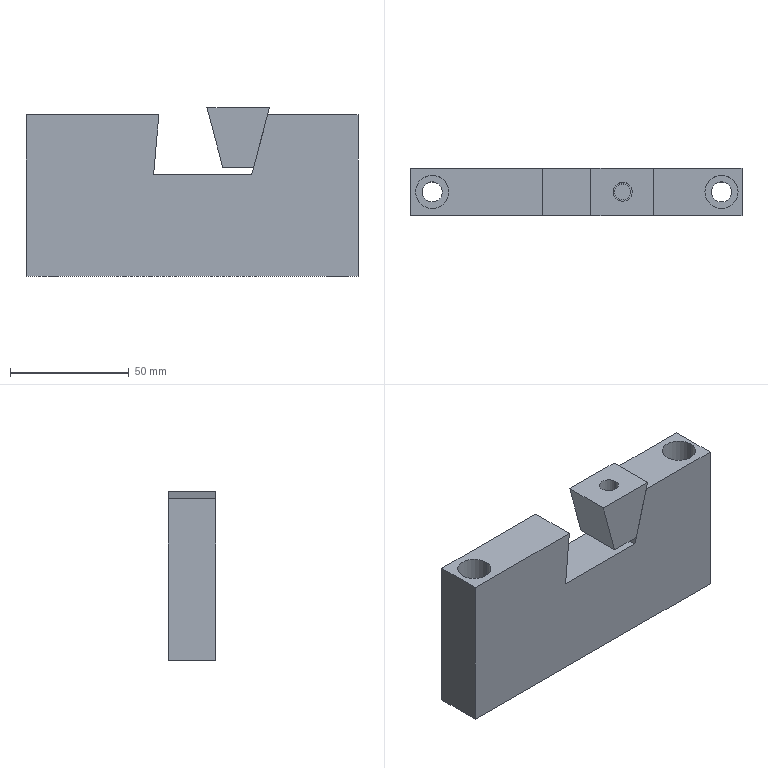Part | Mastercam | 2 solids | 31 faces | box 140 x 20 x 71 mm | volume 164195 mm3 | plane 19 | cylinder 12 | commonest cylinder face diameters 8.5 x4 14 x4 6.8 x2 8 x2
STEP:
#1=CARTESIAN_POINT('',(0.,0.,0.));
#2=DIRECTION('',(0.,0.,1.));
#3=DIRECTION('',(1.,0.,0.));
#4=AXIS2_PLACEMENT_3D('',#1,#2,#3);
#5=CARTESIAN_POINT('',(26.175,18.5,-9.5));
#6=VERTEX_POINT('',#5);
#7=CARTESIAN_POINT('',(18.175,18.5,-9.5));
#8=VERTEX_POINT('',#7);
#9=CARTESIAN_POINT('',(22.175,18.5,-9.5));
#10=DIRECTION('',(0.,0.,-1.));
#11=DIRECTION('',(-1.,0.,0.));
#12=AXIS2_PLACEMENT_3D('',#9,#10,#11);
#13=CIRCLE('',#12,4.);
#14=EDGE_CURVE('',#6,#8,#13,.T.);
#15=ORIENTED_EDGE('',*,*,#14,.F.);
#16=CARTESIAN_POINT('',(22.175,18.5,-9.5));
#17=DIRECTION('',(0.,0.,-1.));
#18=DIRECTION('',(-1.,0.,0.));
#19=AXIS2_PLACEMENT_3D('',#16,#17,#18);
#20=CIRCLE('',#19,4.);
#21=EDGE_CURVE('',#8,#6,#20,.T.);
#22=ORIENTED_EDGE('',*,*,#21,.F.);
#23=EDGE_LOOP('',(#15,#22));
#24=FACE_BOUND('',#23,.T.);
#25=CARTESIAN_POINT('',(15.485,28.5,-9.5));
#26=VERTEX_POINT('',#25);
#27=CARTESIAN_POINT('',(28.476,28.5,-9.5));
#28=VERTEX_POINT('',#27);
#29=CARTESIAN_POINT('',(16.735,28.5,-9.5));
#30=DIRECTION('',(1.,0.,0.));
#31=VECTOR('',#30,1.);
#32=LINE('',#29,#31);
#33=EDGE_CURVE('',#26,#28,#32,.T.);
#34=ORIENTED_EDGE('',*,*,#33,.T.);
#35=CARTESIAN_POINT('',(28.476,8.5,-9.5));
#36=VERTEX_POINT('',#35);
#37=CARTESIAN_POINT('',(28.476,28.5,-9.5));
#38=DIRECTION('',(0.,-1.,0.));
#39=VECTOR('',#38,1.);
#40=LINE('',#37,#39);
#41=EDGE_CURVE('',#28,#36,#40,.T.);
#42=ORIENTED_EDGE('',*,*,#41,.T.);
#43=CARTESIAN_POINT('',(15.485,8.5,-9.5));
#44=VERTEX_POINT('',#43);
#45=CARTESIAN_POINT('',(16.735,8.5,-9.5));
#46=DIRECTION('',(1.,0.,0.));
#47=VECTOR('',#46,1.);
#48=LINE('',#45,#47);
#49=EDGE_CURVE('',#44,#36,#48,.T.);
#50=ORIENTED_EDGE('',*,*,#49,.F.);
#51=CARTESIAN_POINT('',(15.485,28.5,-9.5));
#52=DIRECTION('',(0.,-1.,0.));
#53=VECTOR('',#52,1.);
#54=LINE('',#51,#53);
#55=EDGE_CURVE('',#26,#44,#54,.T.);
#56=ORIENTED_EDGE('',*,*,#55,.F.);
#57=EDGE_LOOP('',(#34,#42,#50,#56));
#58=FACE_OUTER_BOUND('',#57,.T.);
#59=CARTESIAN_POINT('',(16.735,28.5,-9.5));
#60=DIRECTION('',(0.,0.,-1.));
#61=DIRECTION('',(-1.,0.,0.));
#62=AXIS2_PLACEMENT_3D('',#59,#60,#61);
#63=PLANE('',#62);
#64=ADVANCED_FACE('',(#24,#58),#63,.T.);
#65=CARTESIAN_POINT('',(8.786,28.5,15.5));
#66=VERTEX_POINT('',#65);
#67=CARTESIAN_POINT('',(35.175,28.5,15.5));
#68=VERTEX_POINT('',#67);
#69=CARTESIAN_POINT('',(12.68,28.5,15.5));
#70=DIRECTION('',(1.,0.,0.));
#71=VECTOR('',#70,1.);
#72=LINE('',#69,#71);
#73=EDGE_CURVE('',#66,#68,#72,.T.);
#74=ORIENTED_EDGE('',*,*,#73,.T.);
#75=CARTESIAN_POINT('',(28.432,28.5,-9.665));
#76=DIRECTION('',(-0.2588,0.,-0.9659));
#77=VECTOR('',#76,1.);
#78=LINE('',#75,#77);
#79=EDGE_CURVE('',#68,#28,#78,.T.);
#80=ORIENTED_EDGE('',*,*,#79,.T.);
#81=ORIENTED_EDGE('',*,*,#33,.F.);
#82=CARTESIAN_POINT('',(17.578,28.5,-17.312));
#83=DIRECTION('',(-0.2588,0.,0.9659));
#84=VECTOR('',#83,1.);
#85=LINE('',#82,#84);
#86=EDGE_CURVE('',#26,#66,#85,.T.);
#87=ORIENTED_EDGE('',*,*,#86,.T.);
#88=EDGE_LOOP('',(#74,#80,#81,#87));
#89=FACE_OUTER_BOUND('',#88,.T.);
#90=CARTESIAN_POINT('',(-1.,28.5,-4.5));
#91=DIRECTION('',(0.,1.,0.));
#92=DIRECTION('',(0.,0.,1.));
#93=AXIS2_PLACEMENT_3D('',#90,#91,#92);
#94=PLANE('',#93);
#95=ADVANCED_FACE('',(#89),#94,.T.);
#96=CARTESIAN_POINT('',(35.175,8.5,15.5));
#97=VERTEX_POINT('',#96);
#98=CARTESIAN_POINT('',(26.405,8.5,-17.232));
#99=DIRECTION('',(0.2588,0.,0.9659));
#100=VECTOR('',#99,1.);
#101=LINE('',#98,#100);
#102=EDGE_CURVE('',#36,#97,#101,.T.);
#103=ORIENTED_EDGE('',*,*,#102,.T.);
#104=CARTESIAN_POINT('',(8.786,8.5,15.5));
#105=VERTEX_POINT('',#104);
#106=CARTESIAN_POINT('',(12.68,8.5,15.5));
#107=DIRECTION('',(1.,0.,0.));
#108=VECTOR('',#107,1.);
#109=LINE('',#106,#108);
#110=EDGE_CURVE('',#105,#97,#109,.T.);
#111=ORIENTED_EDGE('',*,*,#110,.F.);
#112=CARTESIAN_POINT('',(17.578,8.5,-17.312));
#113=DIRECTION('',(-0.2588,0.,0.9659));
#114=VECTOR('',#113,1.);
#115=LINE('',#112,#114);
#116=EDGE_CURVE('',#44,#105,#115,.T.);
#117=ORIENTED_EDGE('',*,*,#116,.F.);
#118=ORIENTED_EDGE('',*,*,#49,.T.);
#119=EDGE_LOOP('',(#103,#111,#117,#118));
#120=FACE_OUTER_BOUND('',#119,.T.);
#121=CARTESIAN_POINT('',(-1.,8.5,-4.5));
#122=DIRECTION('',(0.,1.,0.));
#123=DIRECTION('',(0.,0.,1.));
#124=AXIS2_PLACEMENT_3D('',#121,#122,#123);
#125=PLANE('',#124);
#126=ADVANCED_FACE('',(#120),#125,.F.);
#127=CARTESIAN_POINT('',(26.175,18.5,15.5));
#128=VERTEX_POINT('',#127);
#129=CARTESIAN_POINT('',(18.175,18.5,15.5));
#130=VERTEX_POINT('',#129);
#131=CARTESIAN_POINT('',(22.175,18.5,15.5));
#132=DIRECTION('',(0.,0.,1.));
#133=DIRECTION('',(-1.,0.,0.));
#134=AXIS2_PLACEMENT_3D('',#131,#132,#133);
#135=CIRCLE('',#134,4.);
#136=EDGE_CURVE('',#128,#130,#135,.T.);
#137=ORIENTED_EDGE('',*,*,#136,.F.);
#138=CARTESIAN_POINT('',(22.175,18.5,15.5));
#139=DIRECTION('',(0.,0.,1.));
#140=DIRECTION('',(-1.,0.,0.));
#141=AXIS2_PLACEMENT_3D('',#138,#139,#140);
#142=CIRCLE('',#141,4.);
#143=EDGE_CURVE('',#130,#128,#142,.T.);
#144=ORIENTED_EDGE('',*,*,#143,.F.);
#145=EDGE_LOOP('',(#137,#144));
#146=FACE_BOUND('',#145,.T.);
#147=ORIENTED_EDGE('',*,*,#110,.T.);
#148=CARTESIAN_POINT('',(35.175,28.5,15.5));
#149=DIRECTION('',(0.,-1.,0.));
#150=VECTOR('',#149,1.);
#151=LINE('',#148,#150);
#152=EDGE_CURVE('',#68,#97,#151,.T.);
#153=ORIENTED_EDGE('',*,*,#152,.F.);
#154=ORIENTED_EDGE('',*,*,#73,.F.);
#155=CARTESIAN_POINT('',(8.786,28.5,15.5));
#156=DIRECTION('',(0.,-1.,0.));
#157=VECTOR('',#156,1.);
#158=LINE('',#155,#157);
#159=EDGE_CURVE('',#66,#105,#158,.T.);
#160=ORIENTED_EDGE('',*,*,#159,.T.);
#161=EDGE_LOOP('',(#147,#153,#154,#160));
#162=FACE_OUTER_BOUND('',#161,.T.);
#163=CARTESIAN_POINT('',(12.68,28.5,15.5));
#164=DIRECTION('',(0.,0.,-1.));
#165=DIRECTION('',(-1.,0.,0.));
#166=AXIS2_PLACEMENT_3D('',#163,#164,#165);
#167=PLANE('',#166);
#168=ADVANCED_FACE('',(#146,#162),#167,.F.);
#169=ORIENTED_EDGE('',*,*,#116,.T.);
#170=ORIENTED_EDGE('',*,*,#159,.F.);
#171=ORIENTED_EDGE('',*,*,#86,.F.);
#172=ORIENTED_EDGE('',*,*,#55,.T.);
#173=EDGE_LOOP('',(#169,#170,#171,#172));
#174=FACE_OUTER_BOUND('',#173,.T.);
#175=CARTESIAN_POINT('',(17.578,28.5,-17.312));
#176=DIRECTION('',(0.9659,0.,0.2588));
#177=DIRECTION('',(0.2588,0.,-0.9659));
#178=AXIS2_PLACEMENT_3D('',#175,#176,#177);
#179=PLANE('',#178);
#180=ADVANCED_FACE('',(#174),#179,.F.);
#181=CARTESIAN_POINT('',(18.175,18.5,-9.5));
#182=DIRECTION('',(0.,0.,1.));
#183=VECTOR('',#182,1.);
#184=LINE('',#181,#183);
#185=EDGE_CURVE('',#8,#130,#184,.T.);
#186=ORIENTED_EDGE('',*,*,#185,.T.);
#187=ORIENTED_EDGE('',*,*,#143,.T.);
#188=CARTESIAN_POINT('',(26.175,18.5,-9.5));
#189=DIRECTION('',(0.,0.,1.));
#190=VECTOR('',#189,1.);
#191=LINE('',#188,#190);
#192=EDGE_CURVE('',#6,#128,#191,.T.);
#193=ORIENTED_EDGE('',*,*,#192,.F.);
#194=ORIENTED_EDGE('',*,*,#14,.T.);
#195=EDGE_LOOP('',(#186,#187,#193,#194));
#196=FACE_OUTER_BOUND('',#195,.T.);
#197=CARTESIAN_POINT('',(22.175,18.5,-17.51));
#198=DIRECTION('',(0.,0.,1.));
#199=DIRECTION('',(0.,1.,0.));
#200=AXIS2_PLACEMENT_3D('',#197,#198,#199);
#201=CYLINDRICAL_SURFACE('',#200,4.);
#202=ADVANCED_FACE('',(#196),#201,.F.);
#203=ORIENTED_EDGE('',*,*,#152,.T.);
#204=ORIENTED_EDGE('',*,*,#102,.F.);
#205=ORIENTED_EDGE('',*,*,#41,.F.);
#206=ORIENTED_EDGE('',*,*,#79,.F.);
#207=EDGE_LOOP('',(#203,#204,#205,#206));
#208=FACE_OUTER_BOUND('',#207,.T.);
#209=CARTESIAN_POINT('',(26.405,31.5,-17.232));
#210=DIRECTION('',(0.9659,0.,-0.2588));
#211=DIRECTION('',(-0.2588,0.,-0.9659));
#212=AXIS2_PLACEMENT_3D('',#209,#210,#211);
#213=PLANE('',#212);
#214=ADVANCED_FACE('',(#208),#213,.T.);
#215=ORIENTED_EDGE('',*,*,#185,.F.);
#216=ORIENTED_EDGE('',*,*,#21,.T.);
#217=ORIENTED_EDGE('',*,*,#192,.T.);
#218=ORIENTED_EDGE('',*,*,#136,.T.);
#219=EDGE_LOOP('',(#215,#216,#217,#218));
#220=FACE_OUTER_BOUND('',#219,.T.);
#221=CARTESIAN_POINT('',(22.175,18.5,-17.51));
#222=DIRECTION('',(0.,0.,1.));
#223=DIRECTION('',(0.,-1.,0.));
#224=AXIS2_PLACEMENT_3D('',#221,#222,#223);
#225=CYLINDRICAL_SURFACE('',#224,4.);
#226=ADVANCED_FACE('',(#220),#225,.F.);
#227=CLOSED_SHELL('',(#64,#95,#126,#168,#180,#202,#214,#226));
#228=MANIFOLD_SOLID_BREP('',#227);
#229=CARTESIAN_POINT('',(18.775,18.5,-12.5));
#230=VERTEX_POINT('',#229);
#231=CARTESIAN_POINT('',(25.575,18.5,-12.5));
#232=VERTEX_POINT('',#231);
#233=CARTESIAN_POINT('',(22.175,18.5,-12.5));
#234=DIRECTION('',(0.,0.,-1.));
#235=DIRECTION('',(-1.,0.,0.));
#236=AXIS2_PLACEMENT_3D('',#233,#234,#235);
#237=CIRCLE('',#236,3.4);
#238=EDGE_CURVE('',#230,#232,#237,.T.);
#239=ORIENTED_EDGE('',*,*,#238,.T.);
#240=CARTESIAN_POINT('',(22.175,18.5,-12.5));
#241=DIRECTION('',(0.,0.,-1.));
#242=DIRECTION('',(-1.,0.,0.));
#243=AXIS2_PLACEMENT_3D('',#240,#241,#242);
#244=CIRCLE('',#243,3.4);
#245=EDGE_CURVE('',#232,#230,#244,.T.);
#246=ORIENTED_EDGE('',*,*,#245,.T.);
#247=EDGE_LOOP('',(#239,#246));
#248=FACE_BOUND('',#247,.T.);
#249=CARTESIAN_POINT('',(27.673,28.5,-12.5));
#250=VERTEX_POINT('',#249);
#251=CARTESIAN_POINT('',(27.673,8.5,-12.5));
#252=VERTEX_POINT('',#251);
#253=CARTESIAN_POINT('',(27.673,58.5,-12.5));
#254=DIRECTION('',(0.,-1.,0.));
#255=VECTOR('',#254,1.);
#256=LINE('',#253,#255);
#257=EDGE_CURVE('',#250,#252,#256,.T.);
#258=ORIENTED_EDGE('',*,*,#257,.F.);
#259=CARTESIAN_POINT('',(-13.683,28.5,-12.5));
#260=VERTEX_POINT('',#259);
#261=CARTESIAN_POINT('',(-20.5,28.5,-12.5));
#262=DIRECTION('',(1.,0.,0.));
#263=VECTOR('',#262,1.);
#264=LINE('',#261,#263);
#265=EDGE_CURVE('',#260,#250,#264,.T.);
#266=ORIENTED_EDGE('',*,*,#265,.F.);
#267=CARTESIAN_POINT('',(-13.683,8.5,-12.5));
#268=VERTEX_POINT('',#267);
#269=CARTESIAN_POINT('',(-13.683,33.5,-12.5));
#270=DIRECTION('',(0.,-1.,0.));
#271=VECTOR('',#270,1.);
#272=LINE('',#269,#271);
#273=EDGE_CURVE('',#260,#268,#272,.T.);
#274=ORIENTED_EDGE('',*,*,#273,.T.);
#275=CARTESIAN_POINT('',(-20.5,8.5,-12.5));
#276=DIRECTION('',(1.,0.,0.));
#277=VECTOR('',#276,1.);
#278=LINE('',#275,#277);
#279=EDGE_CURVE('',#268,#252,#278,.T.);
#280=ORIENTED_EDGE('',*,*,#279,.T.);
#281=EDGE_LOOP('',(#258,#266,#274,#280));
#282=FACE_OUTER_BOUND('',#281,.T.);
#283=CARTESIAN_POINT('',(-20.5,58.5,-12.5));
#284=DIRECTION('',(0.,0.,-1.));
#285=DIRECTION('',(-1.,0.,0.));
#286=AXIS2_PLACEMENT_3D('',#283,#284,#285);
#287=PLANE('',#286);
#288=ADVANCED_FACE('',(#248,#282),#287,.F.);
#289=CARTESIAN_POINT('',(-62.4,18.5,-55.5));
#290=VERTEX_POINT('',#289);
#291=CARTESIAN_POINT('',(-62.4,18.5,-10.5));
#292=VERTEX_POINT('',#291);
#293=CARTESIAN_POINT('',(-62.4,18.5,-55.5));
#294=DIRECTION('',(0.,0.,1.));
#295=VECTOR('',#294,1.);
#296=LINE('',#293,#295);
#297=EDGE_CURVE('',#290,#292,#296,.T.);
#298=ORIENTED_EDGE('',*,*,#297,.T.);
#299=CARTESIAN_POINT('',(-53.9,18.5,-10.5));
#300=VERTEX_POINT('',#299);
#301=CARTESIAN_POINT('',(-58.15,18.5,-10.5));
#302=DIRECTION('',(0.,0.,-1.));
#303=DIRECTION('',(1.,0.,0.));
#304=AXIS2_PLACEMENT_3D('',#301,#302,#303);
#305=CIRCLE('',#304,4.25);
#306=EDGE_CURVE('',#300,#292,#305,.T.);
#307=ORIENTED_EDGE('',*,*,#306,.F.);
#308=CARTESIAN_POINT('',(-53.9,18.5,-55.5));
#309=VERTEX_POINT('',#308);
#310=CARTESIAN_POINT('',(-53.9,18.5,-55.5));
#311=DIRECTION('',(0.,0.,1.));
#312=VECTOR('',#311,1.);
#313=LINE('',#310,#312);
#314=EDGE_CURVE('',#309,#300,#313,.T.);
#315=ORIENTED_EDGE('',*,*,#314,.F.);
#316=CARTESIAN_POINT('',(-58.15,18.5,-55.5));
#317=DIRECTION('',(0.,0.,1.));
#318=DIRECTION('',(1.,0.,0.));
#319=AXIS2_PLACEMENT_3D('',#316,#317,#318);
#320=CIRCLE('',#319,4.25);
#321=EDGE_CURVE('',#290,#309,#320,.T.);
#322=ORIENTED_EDGE('',*,*,#321,.F.);
#323=EDGE_LOOP('',(#298,#307,#315,#322));
#324=FACE_OUTER_BOUND('',#323,.T.);
#325=CARTESIAN_POINT('',(-58.15,18.5,-55.51));
#326=DIRECTION('',(0.,0.,1.));
#327=DIRECTION('',(0.,1.,0.));
#328=AXIS2_PLACEMENT_3D('',#325,#326,#327);
#329=CYLINDRICAL_SURFACE('',#328,4.25);
#330=ADVANCED_FACE('',(#324),#329,.F.);
#331=CARTESIAN_POINT('',(59.6,18.5,-55.5));
#332=VERTEX_POINT('',#331);
#333=CARTESIAN_POINT('',(59.6,18.5,-10.5));
#334=VERTEX_POINT('',#333);
#335=CARTESIAN_POINT('',(59.6,18.5,-55.5));
#336=DIRECTION('',(0.,0.,1.));
#337=VECTOR('',#336,1.);
#338=LINE('',#335,#337);
#339=EDGE_CURVE('',#332,#334,#338,.T.);
#340=ORIENTED_EDGE('',*,*,#339,.T.);
#341=CARTESIAN_POINT('',(68.1,18.5,-10.5));
#342=VERTEX_POINT('',#341);
#343=CARTESIAN_POINT('',(63.85,18.5,-10.5));
#344=DIRECTION('',(0.,0.,-1.));
#345=DIRECTION('',(1.,0.,0.));
#346=AXIS2_PLACEMENT_3D('',#343,#344,#345);
#347=CIRCLE('',#346,4.25);
#348=EDGE_CURVE('',#342,#334,#347,.T.);
#349=ORIENTED_EDGE('',*,*,#348,.F.);
#350=CARTESIAN_POINT('',(68.1,18.5,-55.5));
#351=VERTEX_POINT('',#350);
#352=CARTESIAN_POINT('',(68.1,18.5,-55.5));
#353=DIRECTION('',(0.,0.,1.));
#354=VECTOR('',#353,1.);
#355=LINE('',#352,#354);
#356=EDGE_CURVE('',#351,#342,#355,.T.);
#357=ORIENTED_EDGE('',*,*,#356,.F.);
#358=CARTESIAN_POINT('',(63.85,18.5,-55.5));
#359=DIRECTION('',(0.,0.,1.));
#360=DIRECTION('',(1.,0.,0.));
#361=AXIS2_PLACEMENT_3D('',#358,#359,#360);
#362=CIRCLE('',#361,4.25);
#363=EDGE_CURVE('',#332,#351,#362,.T.);
#364=ORIENTED_EDGE('',*,*,#363,.F.);
#365=EDGE_LOOP('',(#340,#349,#357,#364));
#366=FACE_OUTER_BOUND('',#365,.T.);
#367=CARTESIAN_POINT('',(63.85,18.5,-55.51));
#368=DIRECTION('',(0.,0.,1.));
#369=DIRECTION('',(0.,1.,0.));
#370=AXIS2_PLACEMENT_3D('',#367,#368,#369);
#371=CYLINDRICAL_SURFACE('',#370,4.25);
#372=ADVANCED_FACE('',(#366),#371,.F.);
#373=CARTESIAN_POINT('',(-67.5,8.5,12.5));
#374=VERTEX_POINT('',#373);
#375=CARTESIAN_POINT('',(-67.5,8.5,-55.5));
#376=VERTEX_POINT('',#375);
#377=CARTESIAN_POINT('',(-67.5,8.5,12.5));
#378=DIRECTION('',(0.,0.,-1.));
#379=VECTOR('',#378,1.);
#380=LINE('',#377,#379);
#381=EDGE_CURVE('',#374,#376,#380,.T.);
#382=ORIENTED_EDGE('',*,*,#381,.F.);
#383=CARTESIAN_POINT('',(-67.5,28.5,12.5));
#384=VERTEX_POINT('',#383);
#385=CARTESIAN_POINT('',(-67.5,58.5,12.5));
#386=DIRECTION('',(0.,-1.,0.));
#387=VECTOR('',#386,1.);
#388=LINE('',#385,#387);
#389=EDGE_CURVE('',#384,#374,#388,.T.);
#390=ORIENTED_EDGE('',*,*,#389,.F.);
#391=CARTESIAN_POINT('',(-67.5,28.5,-55.5));
#392=VERTEX_POINT('',#391);
#393=CARTESIAN_POINT('',(-67.5,28.5,12.5));
#394=DIRECTION('',(0.,0.,-1.));
#395=VECTOR('',#394,1.);
#396=LINE('',#393,#395);
#397=EDGE_CURVE('',#384,#392,#396,.T.);
#398=ORIENTED_EDGE('',*,*,#397,.T.);
#399=CARTESIAN_POINT('',(-67.5,58.5,-55.5));
#400=DIRECTION('',(0.,-1.,0.));
#401=VECTOR('',#400,1.);
#402=LINE('',#399,#401);
#403=EDGE_CURVE('',#392,#376,#402,.T.);
#404=ORIENTED_EDGE('',*,*,#403,.T.);
#405=EDGE_LOOP('',(#382,#390,#398,#404));
#406=FACE_OUTER_BOUND('',#405,.T.);
#407=CARTESIAN_POINT('',(-67.5,58.5,12.5));
#408=DIRECTION('',(-1.,0.,0.));
#409=DIRECTION('',(0.,0.,1.));
#410=AXIS2_PLACEMENT_3D('',#407,#408,#409);
#411=PLANE('',#410);
#412=ADVANCED_FACE('',(#406),#411,.T.);
#413=CARTESIAN_POINT('',(-58.15,18.5,-55.5));
#414=DIRECTION('',(0.,0.,1.));
#415=DIRECTION('',(1.,0.,0.));
#416=AXIS2_PLACEMENT_3D('',#413,#414,#415);
#417=CIRCLE('',#416,4.25);
#418=EDGE_CURVE('',#309,#290,#417,.T.);
#419=ORIENTED_EDGE('',*,*,#418,.T.);
#420=ORIENTED_EDGE('',*,*,#321,.T.);
#421=EDGE_LOOP('',(#419,#420));
#422=FACE_BOUND('',#421,.T.);
#423=CARTESIAN_POINT('',(63.85,18.5,-55.5));
#424=DIRECTION('',(0.,0.,1.));
#425=DIRECTION('',(1.,0.,0.));
#426=AXIS2_PLACEMENT_3D('',#423,#424,#425);
#427=CIRCLE('',#426,4.25);
#428=EDGE_CURVE('',#351,#332,#427,.T.);
#429=ORIENTED_EDGE('',*,*,#428,.T.);
#430=ORIENTED_EDGE('',*,*,#363,.T.);
#431=EDGE_LOOP('',(#429,#430));
#432=FACE_BOUND('',#431,.T.);
#433=CARTESIAN_POINT('',(72.5,8.5,-55.5));
#434=VERTEX_POINT('',#433);
#435=CARTESIAN_POINT('',(41.2,8.5,-55.5));
#436=DIRECTION('',(-1.,0.,0.));
#437=VECTOR('',#436,1.);
#438=LINE('',#435,#437);
#439=EDGE_CURVE('',#434,#376,#438,.T.);
#440=ORIENTED_EDGE('',*,*,#439,.T.);
#441=ORIENTED_EDGE('',*,*,#403,.F.);
#442=CARTESIAN_POINT('',(72.5,28.5,-55.5));
#443=VERTEX_POINT('',#442);
#444=CARTESIAN_POINT('',(41.2,28.5,-55.5));
#445=DIRECTION('',(-1.,0.,0.));
#446=VECTOR('',#445,1.);
#447=LINE('',#444,#446);
#448=EDGE_CURVE('',#443,#392,#447,.T.);
#449=ORIENTED_EDGE('',*,*,#448,.F.);
#450=CARTESIAN_POINT('',(72.5,58.5,-55.5));
#451=DIRECTION('',(0.,-1.,0.));
#452=VECTOR('',#451,1.);
#453=LINE('',#450,#452);
#454=EDGE_CURVE('',#443,#434,#453,.T.);
#455=ORIENTED_EDGE('',*,*,#454,.T.);
#456=EDGE_LOOP('',(#440,#441,#449,#455));
#457=FACE_OUTER_BOUND('',#456,.T.);
#458=CARTESIAN_POINT('',(41.2,58.5,-55.5));
#459=DIRECTION('',(0.,0.,1.));
#460=DIRECTION('',(1.,0.,0.));
#461=AXIS2_PLACEMENT_3D('',#458,#459,#460);
#462=PLANE('',#461);
#463=ADVANCED_FACE('',(#422,#432,#457),#462,.F.);
#464=CARTESIAN_POINT('',(72.5,8.5,12.5));
#465=VERTEX_POINT('',#464);
#466=CARTESIAN_POINT('',(72.5,8.5,12.5));
#467=DIRECTION('',(0.,0.,-1.));
#468=VECTOR('',#467,1.);
#469=LINE('',#466,#468);
#470=EDGE_CURVE('',#465,#434,#469,.T.);
#471=ORIENTED_EDGE('',*,*,#470,.T.);
#472=ORIENTED_EDGE('',*,*,#454,.F.);
#473=CARTESIAN_POINT('',(72.5,28.5,12.5));
#474=VERTEX_POINT('',#473);
#475=CARTESIAN_POINT('',(72.5,28.5,12.5));
#476=DIRECTION('',(0.,0.,-1.));
#477=VECTOR('',#476,1.);
#478=LINE('',#475,#477);
#479=EDGE_CURVE('',#474,#443,#478,.T.);
#480=ORIENTED_EDGE('',*,*,#479,.F.);
#481=CARTESIAN_POINT('',(72.5,58.5,12.5));
#482=DIRECTION('',(0.,-1.,0.));
#483=VECTOR('',#482,1.);
#484=LINE('',#481,#483);
#485=EDGE_CURVE('',#474,#465,#484,.T.);
#486=ORIENTED_EDGE('',*,*,#485,.T.);
#487=EDGE_LOOP('',(#471,#472,#480,#486));
#488=FACE_OUTER_BOUND('',#487,.T.);
#489=CARTESIAN_POINT('',(72.5,58.5,12.5));
#490=DIRECTION('',(-1.,0.,0.));
#491=DIRECTION('',(0.,0.,1.));
#492=AXIS2_PLACEMENT_3D('',#489,#490,#491);
#493=PLANE('',#492);
#494=ADVANCED_FACE('',(#488),#493,.F.);
#495=CARTESIAN_POINT('',(56.85,18.5,12.5));
#496=VERTEX_POINT('',#495);
#497=CARTESIAN_POINT('',(70.85,18.5,12.5));
#498=VERTEX_POINT('',#497);
#499=CARTESIAN_POINT('',(63.85,18.5,12.5));
#500=DIRECTION('',(0.,0.,1.));
#501=DIRECTION('',(1.,0.,0.));
#502=AXIS2_PLACEMENT_3D('',#499,#500,#501);
#503=CIRCLE('',#502,7.);
#504=EDGE_CURVE('',#496,#498,#503,.T.);
#505=ORIENTED_EDGE('',*,*,#504,.F.);
#506=CARTESIAN_POINT('',(63.85,18.5,12.5));
#507=DIRECTION('',(0.,0.,1.));
#508=DIRECTION('',(1.,0.,0.));
#509=AXIS2_PLACEMENT_3D('',#506,#507,#508);
#510=CIRCLE('',#509,7.);
#511=EDGE_CURVE('',#498,#496,#510,.T.);
#512=ORIENTED_EDGE('',*,*,#511,.F.);
#513=EDGE_LOOP('',(#505,#512));
#514=FACE_BOUND('',#513,.T.);
#515=CARTESIAN_POINT('',(34.371,8.5,12.5));
#516=VERTEX_POINT('',#515);
#517=CARTESIAN_POINT('',(27.7,8.5,12.5));
#518=DIRECTION('',(1.,0.,0.));
#519=VECTOR('',#518,1.);
#520=LINE('',#517,#519);
#521=EDGE_CURVE('',#516,#465,#520,.T.);
#522=ORIENTED_EDGE('',*,*,#521,.T.);
#523=ORIENTED_EDGE('',*,*,#485,.F.);
#524=CARTESIAN_POINT('',(34.371,28.5,12.5));
#525=VERTEX_POINT('',#524);
#526=CARTESIAN_POINT('',(27.7,28.5,12.5));
#527=DIRECTION('',(1.,0.,0.));
#528=VECTOR('',#527,1.);
#529=LINE('',#526,#528);
#530=EDGE_CURVE('',#525,#474,#529,.T.);
#531=ORIENTED_EDGE('',*,*,#530,.F.);
#532=CARTESIAN_POINT('',(34.371,58.5,12.5));
#533=DIRECTION('',(0.,-1.,0.));
#534=VECTOR('',#533,1.);
#535=LINE('',#532,#534);
#536=EDGE_CURVE('',#525,#516,#535,.T.);
#537=ORIENTED_EDGE('',*,*,#536,.T.);
#538=EDGE_LOOP('',(#522,#523,#531,#537));
#539=FACE_OUTER_BOUND('',#538,.T.);
#540=CARTESIAN_POINT('',(27.7,58.5,12.5));
#541=DIRECTION('',(0.,0.,-1.));
#542=DIRECTION('',(-1.,0.,0.));
#543=AXIS2_PLACEMENT_3D('',#540,#541,#542);
#544=PLANE('',#543);
#545=ADVANCED_FACE('',(#514,#539),#544,.F.);
#546=CARTESIAN_POINT('',(-65.15,18.5,12.5));
#547=VERTEX_POINT('',#546);
#548=CARTESIAN_POINT('',(-51.15,18.5,12.5));
#549=VERTEX_POINT('',#548);
#550=CARTESIAN_POINT('',(-58.15,18.5,12.5));
#551=DIRECTION('',(0.,0.,1.));
#552=DIRECTION('',(1.,0.,0.));
#553=AXIS2_PLACEMENT_3D('',#550,#551,#552);
#554=CIRCLE('',#553,7.);
#555=EDGE_CURVE('',#547,#549,#554,.T.);
#556=ORIENTED_EDGE('',*,*,#555,.F.);
#557=CARTESIAN_POINT('',(-58.15,18.5,12.5));
#558=DIRECTION('',(0.,0.,1.));
#559=DIRECTION('',(1.,0.,0.));
#560=AXIS2_PLACEMENT_3D('',#557,#558,#559);
#561=CIRCLE('',#560,7.);
#562=EDGE_CURVE('',#549,#547,#561,.T.);
#563=ORIENTED_EDGE('',*,*,#562,.F.);
#564=EDGE_LOOP('',(#556,#563));
#565=FACE_BOUND('',#564,.T.);
#566=CARTESIAN_POINT('',(-11.496,8.5,12.5));
#567=VERTEX_POINT('',#566);
#568=CARTESIAN_POINT('',(-20.5,8.5,12.5));
#569=DIRECTION('',(-1.,0.,0.));
#570=VECTOR('',#569,1.);
#571=LINE('',#568,#570);
#572=EDGE_CURVE('',#567,#374,#571,.T.);
#573=ORIENTED_EDGE('',*,*,#572,.F.);
#574=CARTESIAN_POINT('',(-11.496,28.5,12.5));
#575=VERTEX_POINT('',#574);
#576=CARTESIAN_POINT('',(-11.496,58.5,12.5));
#577=DIRECTION('',(0.,-1.,0.));
#578=VECTOR('',#577,1.);
#579=LINE('',#576,#578);
#580=EDGE_CURVE('',#575,#567,#579,.T.);
#581=ORIENTED_EDGE('',*,*,#580,.F.);
#582=CARTESIAN_POINT('',(-20.5,28.5,12.5));
#583=DIRECTION('',(-1.,0.,0.));
#584=VECTOR('',#583,1.);
#585=LINE('',#582,#584);
#586=EDGE_CURVE('',#575,#384,#585,.T.);
#587=ORIENTED_EDGE('',*,*,#586,.T.);
#588=ORIENTED_EDGE('',*,*,#389,.T.);
#589=EDGE_LOOP('',(#573,#581,#587,#588));
#590=FACE_OUTER_BOUND('',#589,.T.);
#591=CARTESIAN_POINT('',(-20.5,58.5,12.5));
#592=DIRECTION('',(0.,0.,1.));
#593=DIRECTION('',(1.,0.,0.));
#594=AXIS2_PLACEMENT_3D('',#591,#592,#593);
#595=PLANE('',#594);
#596=ADVANCED_FACE('',(#565,#590),#595,.T.);
#597=CARTESIAN_POINT('',(-11.504,28.5,12.413));
#598=DIRECTION('',(-0.08716,0.,-0.9962));
#599=VECTOR('',#598,1.);
#600=LINE('',#597,#599);
#601=EDGE_CURVE('',#575,#260,#600,.T.);
#602=ORIENTED_EDGE('',*,*,#601,.T.);
#603=ORIENTED_EDGE('',*,*,#265,.T.);
#604=CARTESIAN_POINT('',(27.902,28.5,-11.642));
#605=DIRECTION('',(0.2588,0.,0.9659));
#606=VECTOR('',#605,1.);
#607=LINE('',#604,#606);
#608=EDGE_CURVE('',#250,#525,#607,.T.);
#609=ORIENTED_EDGE('',*,*,#608,.T.);
#610=ORIENTED_EDGE('',*,*,#530,.T.);
#611=ORIENTED_EDGE('',*,*,#479,.T.);
#612=ORIENTED_EDGE('',*,*,#448,.T.);
#613=ORIENTED_EDGE('',*,*,#397,.F.);
#614=ORIENTED_EDGE('',*,*,#586,.F.);
#615=EDGE_LOOP('',(#602,#603,#609,#610,#611,#612,#613,#614));
#616=FACE_OUTER_BOUND('',#615,.T.);
#617=CARTESIAN_POINT('',(-5.5,28.5,2.5));
#618=DIRECTION('',(0.,1.,0.));
#619=DIRECTION('',(0.,0.,1.));
#620=AXIS2_PLACEMENT_3D('',#617,#618,#619);
#621=PLANE('',#620);
#622=ADVANCED_FACE('',(#616),#621,.T.);
#623=ORIENTED_EDGE('',*,*,#279,.F.);
#624=CARTESIAN_POINT('',(-11.504,8.5,12.413));
#625=DIRECTION('',(-0.08716,0.,-0.9962));
#626=VECTOR('',#625,1.);
#627=LINE('',#624,#626);
#628=EDGE_CURVE('',#567,#268,#627,.T.);
#629=ORIENTED_EDGE('',*,*,#628,.F.);
#630=ORIENTED_EDGE('',*,*,#572,.T.);
#631=ORIENTED_EDGE('',*,*,#381,.T.);
#632=ORIENTED_EDGE('',*,*,#439,.F.);
#633=ORIENTED_EDGE('',*,*,#470,.F.);
#634=ORIENTED_EDGE('',*,*,#521,.F.);
#635=CARTESIAN_POINT('',(27.902,8.5,-11.642));
#636=DIRECTION('',(0.2588,0.,0.9659));
#637=VECTOR('',#636,1.);
#638=LINE('',#635,#637);
#639=EDGE_CURVE('',#252,#516,#638,.T.);
#640=ORIENTED_EDGE('',*,*,#639,.F.);
#641=EDGE_LOOP('',(#623,#629,#630,#631,#632,#633,#634,#640));
#642=FACE_OUTER_BOUND('',#641,.T.);
#643=CARTESIAN_POINT('',(-5.5,8.5,2.5));
#644=DIRECTION('',(0.,1.,0.));
#645=DIRECTION('',(0.,0.,1.));
#646=AXIS2_PLACEMENT_3D('',#643,#644,#645);
#647=PLANE('',#646);
#648=ADVANCED_FACE('',(#642),#647,.F.);
#649=CARTESIAN_POINT('',(18.775,18.5,-34.5));
#650=VERTEX_POINT('',#649);
#651=CARTESIAN_POINT('',(18.775,18.5,-34.5));
#652=DIRECTION('',(0.,0.,1.));
#653=VECTOR('',#652,1.);
#654=LINE('',#651,#653);
#655=EDGE_CURVE('',#650,#230,#654,.T.);
#656=ORIENTED_EDGE('',*,*,#655,.T.);
#657=ORIENTED_EDGE('',*,*,#245,.F.);
#658=CARTESIAN_POINT('',(25.575,18.5,-34.5));
#659=VERTEX_POINT('',#658);
#660=CARTESIAN_POINT('',(25.575,18.5,-34.5));
#661=DIRECTION('',(0.,0.,1.));
#662=VECTOR('',#661,1.);
#663=LINE('',#660,#662);
#664=EDGE_CURVE('',#659,#232,#663,.T.);
#665=ORIENTED_EDGE('',*,*,#664,.F.);
#666=CARTESIAN_POINT('',(22.175,18.5,-34.5));
#667=DIRECTION('',(0.,0.,1.));
#668=DIRECTION('',(1.,0.,0.));
#669=AXIS2_PLACEMENT_3D('',#666,#667,#668);
#670=CIRCLE('',#669,3.4);
#671=EDGE_CURVE('',#650,#659,#670,.T.);
#672=ORIENTED_EDGE('',*,*,#671,.F.);
#673=EDGE_LOOP('',(#656,#657,#665,#672));
#674=FACE_OUTER_BOUND('',#673,.T.);
#675=CARTESIAN_POINT('',(22.175,18.5,-34.5));
#676=DIRECTION('',(0.,0.,1.));
#677=DIRECTION('',(0.,1.,0.));
#678=AXIS2_PLACEMENT_3D('',#675,#676,#677);
#679=CYLINDRICAL_SURFACE('',#678,3.4);
#680=ADVANCED_FACE('',(#674),#679,.F.);
#681=CARTESIAN_POINT('',(22.175,18.5,-34.5));
#682=DIRECTION('',(0.,0.,1.));
#683=DIRECTION('',(1.,0.,0.));
#684=AXIS2_PLACEMENT_3D('',#681,#682,#683);
#685=CIRCLE('',#684,3.4);
#686=EDGE_CURVE('',#659,#650,#685,.T.);
#687=ORIENTED_EDGE('',*,*,#686,.T.);
#688=ORIENTED_EDGE('',*,*,#671,.T.);
#689=EDGE_LOOP('',(#687,#688));
#690=FACE_OUTER_BOUND('',#689,.T.);
#691=CARTESIAN_POINT('',(14.175,18.5,-34.5));
#692=DIRECTION('',(0.,0.,1.));
#693=DIRECTION('',(1.,0.,0.));
#694=AXIS2_PLACEMENT_3D('',#691,#692,#693);
#695=PLANE('',#694);
#696=ADVANCED_FACE('',(#690),#695,.T.);
#697=CARTESIAN_POINT('',(70.85,18.5,-10.5));
#698=VERTEX_POINT('',#697);
#699=CARTESIAN_POINT('',(56.85,18.5,-10.5));
#700=VERTEX_POINT('',#699);
#701=CARTESIAN_POINT('',(63.85,18.5,-10.5));
#702=DIRECTION('',(0.,0.,1.));
#703=DIRECTION('',(1.,0.,0.));
#704=AXIS2_PLACEMENT_3D('',#701,#702,#703);
#705=CIRCLE('',#704,7.);
#706=EDGE_CURVE('',#698,#700,#705,.T.);
#707=ORIENTED_EDGE('',*,*,#706,.T.);
#708=CARTESIAN_POINT('',(63.85,18.5,-10.5));
#709=DIRECTION('',(0.,0.,1.));
#710=DIRECTION('',(1.,0.,0.));
#711=AXIS2_PLACEMENT_3D('',#708,#709,#710);
#712=CIRCLE('',#711,7.);
#713=EDGE_CURVE('',#700,#698,#712,.T.);
#714=ORIENTED_EDGE('',*,*,#713,.T.);
#715=EDGE_LOOP('',(#707,#714));
#716=FACE_OUTER_BOUND('',#715,.T.);
#717=ORIENTED_EDGE('',*,*,#348,.T.);
#718=CARTESIAN_POINT('',(63.85,18.5,-10.5));
#719=DIRECTION('',(0.,0.,-1.));
#720=DIRECTION('',(1.,0.,0.));
#721=AXIS2_PLACEMENT_3D('',#718,#719,#720);
#722=CIRCLE('',#721,4.25);
#723=EDGE_CURVE('',#334,#342,#722,.T.);
#724=ORIENTED_EDGE('',*,*,#723,.T.);
#725=EDGE_LOOP('',(#717,#724));
#726=FACE_BOUND('',#725,.T.);
#727=CARTESIAN_POINT('',(63.85,18.5,-10.5));
#728=DIRECTION('',(0.,0.,1.));
#729=DIRECTION('',(1.,0.,0.));
#730=AXIS2_PLACEMENT_3D('',#727,#728,#729);
#731=PLANE('',#730);
#732=ADVANCED_FACE('',(#716,#726),#731,.T.);
#733=CARTESIAN_POINT('',(56.85,18.5,-10.5));
#734=DIRECTION('',(0.,0.,1.));
#735=VECTOR('',#734,1.);
#736=LINE('',#733,#735);
#737=EDGE_CURVE('',#700,#496,#736,.T.);
#738=ORIENTED_EDGE('',*,*,#737,.T.);
#739=ORIENTED_EDGE('',*,*,#504,.T.);
#740=CARTESIAN_POINT('',(70.85,18.5,-10.5));
#741=DIRECTION('',(0.,0.,1.));
#742=VECTOR('',#741,1.);
#743=LINE('',#740,#742);
#744=EDGE_CURVE('',#698,#498,#743,.T.);
#745=ORIENTED_EDGE('',*,*,#744,.F.);
#746=ORIENTED_EDGE('',*,*,#713,.F.);
#747=EDGE_LOOP('',(#738,#739,#745,#746));
#748=FACE_OUTER_BOUND('',#747,.T.);
#749=CARTESIAN_POINT('',(63.85,18.5,-10.5));
#750=DIRECTION('',(0.,0.,1.));
#751=DIRECTION('',(0.,1.,0.));
#752=AXIS2_PLACEMENT_3D('',#749,#750,#751);
#753=CYLINDRICAL_SURFACE('',#752,7.);
#754=ADVANCED_FACE('',(#748),#753,.F.);
#755=CARTESIAN_POINT('',(-51.15,18.5,-10.5));
#756=VERTEX_POINT('',#755);
#757=CARTESIAN_POINT('',(-65.15,18.5,-10.5));
#758=VERTEX_POINT('',#757);
#759=CARTESIAN_POINT('',(-58.15,18.5,-10.5));
#760=DIRECTION('',(0.,0.,1.));
#761=DIRECTION('',(1.,0.,0.));
#762=AXIS2_PLACEMENT_3D('',#759,#760,#761);
#763=CIRCLE('',#762,7.);
#764=EDGE_CURVE('',#756,#758,#763,.T.);
#765=ORIENTED_EDGE('',*,*,#764,.T.);
#766=CARTESIAN_POINT('',(-58.15,18.5,-10.5));
#767=DIRECTION('',(0.,0.,1.));
#768=DIRECTION('',(1.,0.,0.));
#769=AXIS2_PLACEMENT_3D('',#766,#767,#768);
#770=CIRCLE('',#769,7.);
#771=EDGE_CURVE('',#758,#756,#770,.T.);
#772=ORIENTED_EDGE('',*,*,#771,.T.);
#773=EDGE_LOOP('',(#765,#772));
#774=FACE_OUTER_BOUND('',#773,.T.);
#775=ORIENTED_EDGE('',*,*,#306,.T.);
#776=CARTESIAN_POINT('',(-58.15,18.5,-10.5));
#777=DIRECTION('',(0.,0.,-1.));
#778=DIRECTION('',(1.,0.,0.));
#779=AXIS2_PLACEMENT_3D('',#776,#777,#778);
#780=CIRCLE('',#779,4.25);
#781=EDGE_CURVE('',#292,#300,#780,.T.);
#782=ORIENTED_EDGE('',*,*,#781,.T.);
#783=EDGE_LOOP('',(#775,#782));
#784=FACE_BOUND('',#783,.T.);
#785=CARTESIAN_POINT('',(-58.15,18.5,-10.5));
#786=DIRECTION('',(0.,0.,1.));
#787=DIRECTION('',(1.,0.,0.));
#788=AXIS2_PLACEMENT_3D('',#785,#786,#787);
#789=PLANE('',#788);
#790=ADVANCED_FACE('',(#774,#784),#789,.T.);
#791=CARTESIAN_POINT('',(-65.15,18.5,-10.5));
#792=DIRECTION('',(0.,0.,1.));
#793=VECTOR('',#792,1.);
#794=LINE('',#791,#793);
#795=EDGE_CURVE('',#758,#547,#794,.T.);
#796=ORIENTED_EDGE('',*,*,#795,.T.);
#797=ORIENTED_EDGE('',*,*,#555,.T.);
#798=CARTESIAN_POINT('',(-51.15,18.5,-10.5));
#799=DIRECTION('',(0.,0.,1.));
#800=VECTOR('',#799,1.);
#801=LINE('',#798,#800);
#802=EDGE_CURVE('',#756,#549,#801,.T.);
#803=ORIENTED_EDGE('',*,*,#802,.F.);
#804=ORIENTED_EDGE('',*,*,#771,.F.);
#805=EDGE_LOOP('',(#796,#797,#803,#804));
#806=FACE_OUTER_BOUND('',#805,.T.);
#807=CARTESIAN_POINT('',(-58.15,18.5,-10.5));
#808=DIRECTION('',(0.,0.,1.));
#809=DIRECTION('',(0.,1.,0.));
#810=AXIS2_PLACEMENT_3D('',#807,#808,#809);
#811=CYLINDRICAL_SURFACE('',#810,7.);
#812=ADVANCED_FACE('',(#806),#811,.F.);
#813=ORIENTED_EDGE('',*,*,#639,.T.);
#814=ORIENTED_EDGE('',*,*,#536,.F.);
#815=ORIENTED_EDGE('',*,*,#608,.F.);
#816=ORIENTED_EDGE('',*,*,#257,.T.);
#817=EDGE_LOOP('',(#813,#814,#815,#816));
#818=FACE_OUTER_BOUND('',#817,.T.);
#819=CARTESIAN_POINT('',(27.902,43.5,-11.642));
#820=DIRECTION('',(0.9659,0.,-0.2588));
#821=DIRECTION('',(-0.2588,0.,-0.9659));
#822=AXIS2_PLACEMENT_3D('',#819,#820,#821);
#823=PLANE('',#822);
#824=ADVANCED_FACE('',(#818),#823,.F.);
#825=ORIENTED_EDGE('',*,*,#628,.T.);
#826=ORIENTED_EDGE('',*,*,#273,.F.);
#827=ORIENTED_EDGE('',*,*,#601,.F.);
#828=ORIENTED_EDGE('',*,*,#580,.T.);
#829=EDGE_LOOP('',(#825,#826,#827,#828));
#830=FACE_OUTER_BOUND('',#829,.T.);
#831=CARTESIAN_POINT('',(-11.504,33.5,12.413));
#832=DIRECTION('',(-0.9962,0.,0.08716));
#833=DIRECTION('',(0.08716,0.,0.9962));
#834=AXIS2_PLACEMENT_3D('',#831,#832,#833);
#835=PLANE('',#834);
#836=ADVANCED_FACE('',(#830),#835,.F.);
#837=ORIENTED_EDGE('',*,*,#297,.F.);
#838=ORIENTED_EDGE('',*,*,#418,.F.);
#839=ORIENTED_EDGE('',*,*,#314,.T.);
#840=ORIENTED_EDGE('',*,*,#781,.F.);
#841=EDGE_LOOP('',(#837,#838,#839,#840));
#842=FACE_OUTER_BOUND('',#841,.T.);
#843=CARTESIAN_POINT('',(-58.15,18.5,-55.51));
#844=DIRECTION('',(0.,0.,1.));
#845=DIRECTION('',(0.,-1.,0.));
#846=AXIS2_PLACEMENT_3D('',#843,#844,#845);
#847=CYLINDRICAL_SURFACE('',#846,4.25);
#848=ADVANCED_FACE('',(#842),#847,.F.);
#849=ORIENTED_EDGE('',*,*,#339,.F.);
#850=ORIENTED_EDGE('',*,*,#428,.F.);
#851=ORIENTED_EDGE('',*,*,#356,.T.);
#852=ORIENTED_EDGE('',*,*,#723,.F.);
#853=EDGE_LOOP('',(#849,#850,#851,#852));
#854=FACE_OUTER_BOUND('',#853,.T.);
#855=CARTESIAN_POINT('',(63.85,18.5,-55.51));
#856=DIRECTION('',(0.,0.,1.));
#857=DIRECTION('',(0.,-1.,0.));
#858=AXIS2_PLACEMENT_3D('',#855,#856,#857);
#859=CYLINDRICAL_SURFACE('',#858,4.25);
#860=ADVANCED_FACE('',(#854),#859,.F.);
#861=ORIENTED_EDGE('',*,*,#655,.F.);
#862=ORIENTED_EDGE('',*,*,#686,.F.);
#863=ORIENTED_EDGE('',*,*,#664,.T.);
#864=ORIENTED_EDGE('',*,*,#238,.F.);
#865=EDGE_LOOP('',(#861,#862,#863,#864));
#866=FACE_OUTER_BOUND('',#865,.T.);
#867=CARTESIAN_POINT('',(22.175,18.5,-34.5));
#868=DIRECTION('',(0.,0.,1.));
#869=DIRECTION('',(0.,-1.,0.));
#870=AXIS2_PLACEMENT_3D('',#867,#868,#869);
#871=CYLINDRICAL_SURFACE('',#870,3.4);
#872=ADVANCED_FACE('',(#866),#871,.F.);
#873=ORIENTED_EDGE('',*,*,#737,.F.);
#874=ORIENTED_EDGE('',*,*,#706,.F.);
#875=ORIENTED_EDGE('',*,*,#744,.T.);
#876=ORIENTED_EDGE('',*,*,#511,.T.);
#877=EDGE_LOOP('',(#873,#874,#875,#876));
#878=FACE_OUTER_BOUND('',#877,.T.);
#879=CARTESIAN_POINT('',(63.85,18.5,-10.5));
#880=DIRECTION('',(0.,0.,1.));
#881=DIRECTION('',(0.,-1.,0.));
#882=AXIS2_PLACEMENT_3D('',#879,#880,#881);
#883=CYLINDRICAL_SURFACE('',#882,7.);
#884=ADVANCED_FACE('',(#878),#883,.F.);
#885=ORIENTED_EDGE('',*,*,#795,.F.);
#886=ORIENTED_EDGE('',*,*,#764,.F.);
#887=ORIENTED_EDGE('',*,*,#802,.T.);
#888=ORIENTED_EDGE('',*,*,#562,.T.);
#889=EDGE_LOOP('',(#885,#886,#887,#888));
#890=FACE_OUTER_BOUND('',#889,.T.);
#891=CARTESIAN_POINT('',(-58.15,18.5,-10.5));
#892=DIRECTION('',(0.,0.,1.));
#893=DIRECTION('',(0.,-1.,0.));
#894=AXIS2_PLACEMENT_3D('',#891,#892,#893);
#895=CYLINDRICAL_SURFACE('',#894,7.);
#896=ADVANCED_FACE('',(#890),#895,.F.);
#897=CLOSED_SHELL('',(#288,#330,#372,#412,#463,#494,#545,#596,#622,#648,#680,#696,#732,#754,#790,#812,#824,#836,#848,#860,#872,#884,#896));
#898=MANIFOLD_SOLID_BREP('',#897);
#899=(LENGTH_UNIT()NAMED_UNIT(*)SI_UNIT(.MILLI.,.METRE.));
#900=UNCERTAINTY_MEASURE_WITH_UNIT(LENGTH_MEASURE(0.005),#899,'','');
#901=(NAMED_UNIT(*)PLANE_ANGLE_UNIT()SI_UNIT($,.RADIAN.));
#902=(GEOMETRIC_REPRESENTATION_CONTEXT(3)GLOBAL_UNCERTAINTY_ASSIGNED_CONTEXT((#900))GLOBAL_UNIT_ASSIGNED_CONTEXT((#899,#901))REPRESENTATION_CONTEXT('',''));
#903=ADVANCED_BREP_SHAPE_REPRESENTATION('',(#4,#228,#898),#902);